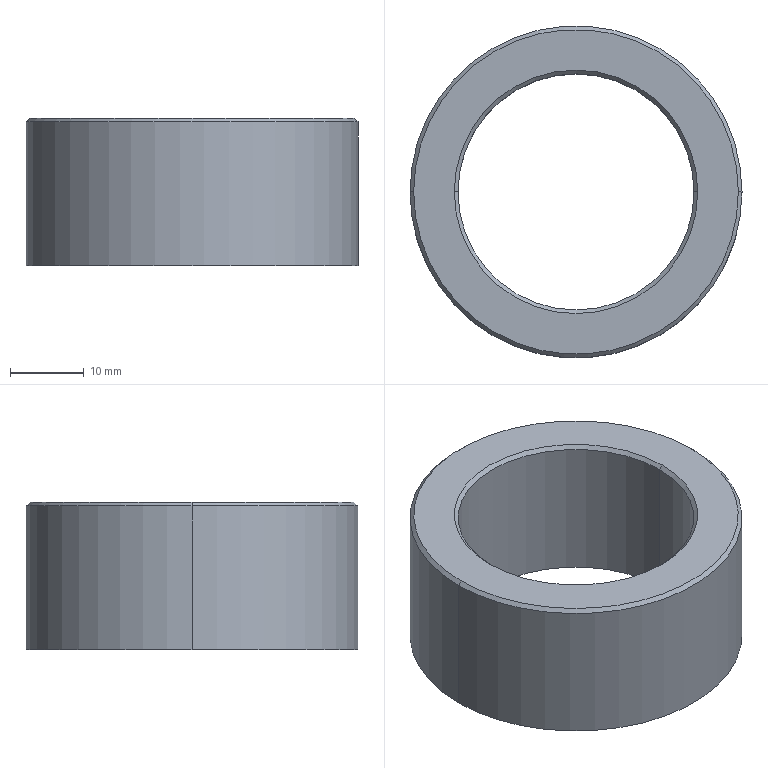Part | SolidWorks | features Chamfer 2, Extrusion 1, ICE 1 | 1 solid | 10 faces | box 45 x 45 x 20 mm | volume 15693 mm3 | cone 4 | cylinder 4 | plane 2 | commonest cylinder face diameters 32 x2 45 x2
STEP:
#1=CARTESIAN_POINT('',(22.,0.,20.));
#2=VERTEX_POINT('',#1);
#3=CARTESIAN_POINT('',(-22.,0.,20.));
#4=VERTEX_POINT('',#3);
#5=CARTESIAN_POINT('',(0.,0.,20.));
#6=DIRECTION('',(0.,0.,1.));
#7=DIRECTION('',(1.,0.,0.));
#8=AXIS2_PLACEMENT_3D('',#5,#6,#7);
#9=CIRCLE('',#8,22.);
#10=EDGE_CURVE('',#2,#4,#9,.T.);
#11=ORIENTED_EDGE('',*,*,#10,.F.);
#12=CARTESIAN_POINT('',(22.5,0.,19.5));
#13=VERTEX_POINT('',#12);
#14=CARTESIAN_POINT('',(22.,0.,20.));
#15=DIRECTION('',(0.7071,0.,-0.7071));
#16=VECTOR('',#15,1000.);
#17=LINE('',#14,#16);
#18=EDGE_CURVE('',#2,#13,#17,.T.);
#19=ORIENTED_EDGE('',*,*,#18,.T.);
#20=CARTESIAN_POINT('',(-22.5,0.,19.5));
#21=VERTEX_POINT('',#20);
#22=CARTESIAN_POINT('',(0.,0.,19.5));
#23=DIRECTION('',(0.,0.,-1.));
#24=DIRECTION('',(1.,0.,0.));
#25=AXIS2_PLACEMENT_3D('',#22,#23,#24);
#26=CIRCLE('',#25,22.5);
#27=EDGE_CURVE('',#21,#13,#26,.T.);
#28=ORIENTED_EDGE('',*,*,#27,.F.);
#29=CARTESIAN_POINT('',(-22.,0.,20.));
#30=DIRECTION('',(-0.7071,0.,-0.7071));
#31=VECTOR('',#30,1000.);
#32=LINE('',#29,#31);
#33=EDGE_CURVE('',#4,#21,#32,.T.);
#34=ORIENTED_EDGE('',*,*,#33,.F.);
#35=EDGE_LOOP('',(#11,#19,#28,#34));
#36=FACE_OUTER_BOUND('',#35,.T.);
#37=CARTESIAN_POINT('',(0.,0.,20.));
#38=DIRECTION('',(0.,0.,-1.));
#39=DIRECTION('',(-1.,0.,0.));
#40=AXIS2_PLACEMENT_3D('',#37,#38,#39);
#41=CONICAL_SURFACE('',#40,22.,0.7854);
#42=ADVANCED_FACE('',(#36),#41,.T.);
#43=CARTESIAN_POINT('',(-16.,0.,19.5));
#44=VERTEX_POINT('',#43);
#45=CARTESIAN_POINT('',(16.,0.,19.5));
#46=VERTEX_POINT('',#45);
#47=CARTESIAN_POINT('',(0.,0.,19.5));
#48=DIRECTION('',(0.,0.,1.));
#49=DIRECTION('',(1.,0.,0.));
#50=AXIS2_PLACEMENT_3D('',#47,#48,#49);
#51=CIRCLE('',#50,16.);
#52=EDGE_CURVE('',#44,#46,#51,.T.);
#53=ORIENTED_EDGE('',*,*,#52,.F.);
#54=CARTESIAN_POINT('',(-16.5,0.,20.));
#55=VERTEX_POINT('',#54);
#56=CARTESIAN_POINT('',(-16.,0.,19.5));
#57=DIRECTION('',(-0.7071,0.,0.7071));
#58=VECTOR('',#57,1000.);
#59=LINE('',#56,#58);
#60=EDGE_CURVE('',#44,#55,#59,.T.);
#61=ORIENTED_EDGE('',*,*,#60,.T.);
#62=CARTESIAN_POINT('',(16.5,0.,20.));
#63=VERTEX_POINT('',#62);
#64=CARTESIAN_POINT('',(0.,0.,20.));
#65=DIRECTION('',(0.,0.,-1.));
#66=DIRECTION('',(1.,0.,0.));
#67=AXIS2_PLACEMENT_3D('',#64,#65,#66);
#68=CIRCLE('',#67,16.5);
#69=EDGE_CURVE('',#63,#55,#68,.T.);
#70=ORIENTED_EDGE('',*,*,#69,.F.);
#71=CARTESIAN_POINT('',(16.,0.,19.5));
#72=DIRECTION('',(0.7071,0.,0.7071));
#73=VECTOR('',#72,1000.);
#74=LINE('',#71,#73);
#75=EDGE_CURVE('',#46,#63,#74,.T.);
#76=ORIENTED_EDGE('',*,*,#75,.F.);
#77=EDGE_LOOP('',(#53,#61,#70,#76));
#78=FACE_OUTER_BOUND('',#77,.T.);
#79=CARTESIAN_POINT('',(0.,0.,19.5));
#80=DIRECTION('',(0.,0.,1.));
#81=DIRECTION('',(1.,0.,0.));
#82=AXIS2_PLACEMENT_3D('',#79,#80,#81);
#83=CONICAL_SURFACE('',#82,16.,0.7854);
#84=ADVANCED_FACE('',(#78),#83,.F.);
#85=CARTESIAN_POINT('',(-16.,0.,0.));
#86=VERTEX_POINT('',#85);
#87=CARTESIAN_POINT('',(16.,0.,0.));
#88=VERTEX_POINT('',#87);
#89=CARTESIAN_POINT('',(0.,0.,0.));
#90=DIRECTION('',(0.,0.,1.));
#91=DIRECTION('',(1.,0.,0.));
#92=AXIS2_PLACEMENT_3D('',#89,#90,#91);
#93=CIRCLE('',#92,16.);
#94=EDGE_CURVE('',#86,#88,#93,.T.);
#95=ORIENTED_EDGE('',*,*,#94,.F.);
#96=CARTESIAN_POINT('',(-16.,0.,0.));
#97=DIRECTION('',(0.,0.,1.));
#98=VECTOR('',#97,1000.);
#99=LINE('',#96,#98);
#100=EDGE_CURVE('',#86,#44,#99,.T.);
#101=ORIENTED_EDGE('',*,*,#100,.T.);
#102=ORIENTED_EDGE('',*,*,#52,.T.);
#103=CARTESIAN_POINT('',(16.,0.,0.));
#104=DIRECTION('',(0.,0.,1.));
#105=VECTOR('',#104,1000.);
#106=LINE('',#103,#105);
#107=EDGE_CURVE('',#88,#46,#106,.T.);
#108=ORIENTED_EDGE('',*,*,#107,.F.);
#109=EDGE_LOOP('',(#95,#101,#102,#108));
#110=FACE_OUTER_BOUND('',#109,.T.);
#111=CARTESIAN_POINT('',(0.,0.,0.));
#112=DIRECTION('',(0.,0.,1.));
#113=DIRECTION('',(1.,0.,0.));
#114=AXIS2_PLACEMENT_3D('',#111,#112,#113);
#115=CYLINDRICAL_SURFACE('',#114,16.);
#116=ADVANCED_FACE('',(#110),#115,.F.);
#117=ORIENTED_EDGE('',*,*,#27,.T.);
#118=CARTESIAN_POINT('',(22.5,0.,0.));
#119=VERTEX_POINT('',#118);
#120=CARTESIAN_POINT('',(22.5,0.,20.));
#121=DIRECTION('',(0.,0.,-1.));
#122=VECTOR('',#121,1000.);
#123=LINE('',#120,#122);
#124=EDGE_CURVE('',#13,#119,#123,.T.);
#125=ORIENTED_EDGE('',*,*,#124,.T.);
#126=CARTESIAN_POINT('',(-22.5,0.,0.));
#127=VERTEX_POINT('',#126);
#128=CARTESIAN_POINT('',(0.,0.,0.));
#129=DIRECTION('',(0.,0.,1.));
#130=DIRECTION('',(1.,0.,0.));
#131=AXIS2_PLACEMENT_3D('',#128,#129,#130);
#132=CIRCLE('',#131,22.5);
#133=EDGE_CURVE('',#119,#127,#132,.T.);
#134=ORIENTED_EDGE('',*,*,#133,.T.);
#135=CARTESIAN_POINT('',(-22.5,0.,20.));
#136=DIRECTION('',(0.,0.,-1.));
#137=VECTOR('',#136,1000.);
#138=LINE('',#135,#137);
#139=EDGE_CURVE('',#21,#127,#138,.T.);
#140=ORIENTED_EDGE('',*,*,#139,.F.);
#141=EDGE_LOOP('',(#117,#125,#134,#140));
#142=FACE_OUTER_BOUND('',#141,.T.);
#143=CARTESIAN_POINT('',(0.,0.,20.));
#144=DIRECTION('',(0.,0.,-1.));
#145=DIRECTION('',(-1.,0.,0.));
#146=AXIS2_PLACEMENT_3D('',#143,#144,#145);
#147=CYLINDRICAL_SURFACE('',#146,22.5);
#148=ADVANCED_FACE('',(#142),#147,.T.);
#149=ORIENTED_EDGE('',*,*,#124,.F.);
#150=CARTESIAN_POINT('',(0.,0.,19.5));
#151=DIRECTION('',(0.,0.,-1.));
#152=DIRECTION('',(1.,0.,0.));
#153=AXIS2_PLACEMENT_3D('',#150,#151,#152);
#154=CIRCLE('',#153,22.5);
#155=EDGE_CURVE('',#13,#21,#154,.T.);
#156=ORIENTED_EDGE('',*,*,#155,.T.);
#157=ORIENTED_EDGE('',*,*,#139,.T.);
#158=CARTESIAN_POINT('',(0.,0.,0.));
#159=DIRECTION('',(0.,0.,1.));
#160=DIRECTION('',(1.,0.,0.));
#161=AXIS2_PLACEMENT_3D('',#158,#159,#160);
#162=CIRCLE('',#161,22.5);
#163=EDGE_CURVE('',#127,#119,#162,.T.);
#164=ORIENTED_EDGE('',*,*,#163,.T.);
#165=EDGE_LOOP('',(#149,#156,#157,#164));
#166=FACE_OUTER_BOUND('',#165,.T.);
#167=CARTESIAN_POINT('',(0.,0.,20.));
#168=DIRECTION('',(0.,0.,-1.));
#169=DIRECTION('',(-1.,0.,0.));
#170=AXIS2_PLACEMENT_3D('',#167,#168,#169);
#171=CYLINDRICAL_SURFACE('',#170,22.5);
#172=ADVANCED_FACE('',(#166),#171,.T.);
#173=CARTESIAN_POINT('',(0.,0.,20.));
#174=DIRECTION('',(0.,0.,1.));
#175=DIRECTION('',(1.,0.,0.));
#176=AXIS2_PLACEMENT_3D('',#173,#174,#175);
#177=CIRCLE('',#176,22.);
#178=EDGE_CURVE('',#4,#2,#177,.T.);
#179=ORIENTED_EDGE('',*,*,#178,.T.);
#180=ORIENTED_EDGE('',*,*,#10,.T.);
#181=EDGE_LOOP('',(#179,#180));
#182=FACE_OUTER_BOUND('',#181,.T.);
#183=ORIENTED_EDGE('',*,*,#69,.T.);
#184=CARTESIAN_POINT('',(0.,0.,20.));
#185=DIRECTION('',(0.,0.,-1.));
#186=DIRECTION('',(1.,0.,0.));
#187=AXIS2_PLACEMENT_3D('',#184,#185,#186);
#188=CIRCLE('',#187,16.5);
#189=EDGE_CURVE('',#55,#63,#188,.T.);
#190=ORIENTED_EDGE('',*,*,#189,.T.);
#191=EDGE_LOOP('',(#183,#190));
#192=FACE_BOUND('',#191,.T.);
#193=CARTESIAN_POINT('',(0.,0.,20.));
#194=DIRECTION('',(0.,0.,1.));
#195=DIRECTION('',(1.,0.,0.));
#196=AXIS2_PLACEMENT_3D('',#193,#194,#195);
#197=PLANE('',#196);
#198=ADVANCED_FACE('',(#182,#192),#197,.T.);
#199=CARTESIAN_POINT('',(0.,0.,0.));
#200=DIRECTION('',(0.,0.,1.));
#201=DIRECTION('',(1.,0.,0.));
#202=AXIS2_PLACEMENT_3D('',#199,#200,#201);
#203=CIRCLE('',#202,16.);
#204=EDGE_CURVE('',#88,#86,#203,.T.);
#205=ORIENTED_EDGE('',*,*,#204,.T.);
#206=ORIENTED_EDGE('',*,*,#94,.T.);
#207=EDGE_LOOP('',(#205,#206));
#208=FACE_BOUND('',#207,.T.);
#209=ORIENTED_EDGE('',*,*,#163,.F.);
#210=ORIENTED_EDGE('',*,*,#133,.F.);
#211=EDGE_LOOP('',(#209,#210));
#212=FACE_OUTER_BOUND('',#211,.T.);
#213=CARTESIAN_POINT('',(0.,0.,0.));
#214=DIRECTION('',(0.,0.,1.));
#215=DIRECTION('',(1.,0.,0.));
#216=AXIS2_PLACEMENT_3D('',#213,#214,#215);
#217=PLANE('',#216);
#218=ADVANCED_FACE('',(#208,#212),#217,.F.);
#219=ORIENTED_EDGE('',*,*,#100,.F.);
#220=ORIENTED_EDGE('',*,*,#204,.F.);
#221=ORIENTED_EDGE('',*,*,#107,.T.);
#222=CARTESIAN_POINT('',(0.,0.,19.5));
#223=DIRECTION('',(0.,0.,1.));
#224=DIRECTION('',(1.,0.,0.));
#225=AXIS2_PLACEMENT_3D('',#222,#223,#224);
#226=CIRCLE('',#225,16.);
#227=EDGE_CURVE('',#46,#44,#226,.T.);
#228=ORIENTED_EDGE('',*,*,#227,.T.);
#229=EDGE_LOOP('',(#219,#220,#221,#228));
#230=FACE_OUTER_BOUND('',#229,.T.);
#231=CARTESIAN_POINT('',(0.,0.,0.));
#232=DIRECTION('',(0.,0.,1.));
#233=DIRECTION('',(1.,0.,0.));
#234=AXIS2_PLACEMENT_3D('',#231,#232,#233);
#235=CYLINDRICAL_SURFACE('',#234,16.);
#236=ADVANCED_FACE('',(#230),#235,.F.);
#237=ORIENTED_EDGE('',*,*,#60,.F.);
#238=ORIENTED_EDGE('',*,*,#227,.F.);
#239=ORIENTED_EDGE('',*,*,#75,.T.);
#240=ORIENTED_EDGE('',*,*,#189,.F.);
#241=EDGE_LOOP('',(#237,#238,#239,#240));
#242=FACE_OUTER_BOUND('',#241,.T.);
#243=CARTESIAN_POINT('',(0.,0.,19.5));
#244=DIRECTION('',(0.,0.,1.));
#245=DIRECTION('',(1.,0.,0.));
#246=AXIS2_PLACEMENT_3D('',#243,#244,#245);
#247=CONICAL_SURFACE('',#246,16.,0.7854);
#248=ADVANCED_FACE('',(#242),#247,.F.);
#249=ORIENTED_EDGE('',*,*,#18,.F.);
#250=ORIENTED_EDGE('',*,*,#178,.F.);
#251=ORIENTED_EDGE('',*,*,#33,.T.);
#252=ORIENTED_EDGE('',*,*,#155,.F.);
#253=EDGE_LOOP('',(#249,#250,#251,#252));
#254=FACE_OUTER_BOUND('',#253,.T.);
#255=CARTESIAN_POINT('',(0.,0.,20.));
#256=DIRECTION('',(0.,0.,-1.));
#257=DIRECTION('',(-1.,0.,0.));
#258=AXIS2_PLACEMENT_3D('',#255,#256,#257);
#259=CONICAL_SURFACE('',#258,22.,0.7854);
#260=ADVANCED_FACE('',(#254),#259,.T.);
#261=CLOSED_SHELL('',(#42,#84,#116,#148,#172,#198,#218,#236,#248,#260));
#262=MANIFOLD_SOLID_BREP('',#261);
#263=CARTESIAN_POINT('',(0.,0.,0.));
#264=DIRECTION('',(0.,0.,1.));
#265=DIRECTION('',(1.,0.,0.));
#266=AXIS2_PLACEMENT_3D('',#263,#264,#265);
#267=(LENGTH_UNIT()NAMED_UNIT(*)SI_UNIT(.MILLI.,.METRE.));
#268=UNCERTAINTY_MEASURE_WITH_UNIT(LENGTH_MEASURE(0.00001),#267,'','');
#269=(NAMED_UNIT(*)PLANE_ANGLE_UNIT()SI_UNIT($,.RADIAN.));
#270=(NAMED_UNIT(*)SI_UNIT($,.STERADIAN.)SOLID_ANGLE_UNIT());
#271=(GEOMETRIC_REPRESENTATION_CONTEXT(3)GLOBAL_UNCERTAINTY_ASSIGNED_CONTEXT((#268))GLOBAL_UNIT_ASSIGNED_CONTEXT((#267,#269,#270))REPRESENTATION_CONTEXT('',''));
#272=ADVANCED_BREP_SHAPE_REPRESENTATION('',(#262,#266),#271);